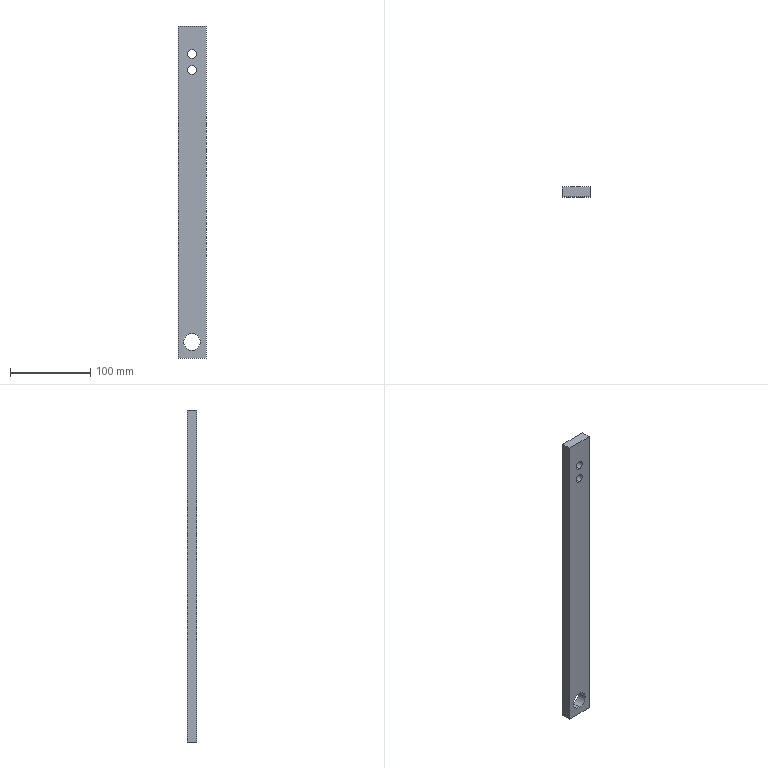Part | SolidWorks | features Extrusion 1, ICE 1 | 1 solid | 12 faces | box 35 x 12 x 415 mm | volume 167863 mm3 | cylinder 6 | plane 6 | commonest cylinder face diameters 11 x4 21 x2
STEP:
#1=CARTESIAN_POINT('',(0.,-6.,178.));
#2=VERTEX_POINT('',#1);
#3=CARTESIAN_POINT('',(0.,-6.,167.));
#4=VERTEX_POINT('',#3);
#5=CARTESIAN_POINT('',(0.,-6.,172.5));
#6=DIRECTION('',(0.,-1.,0.));
#7=DIRECTION('',(0.,0.,1.));
#8=AXIS2_PLACEMENT_3D('',#5,#6,#7);
#9=CIRCLE('',#8,5.5);
#10=EDGE_CURVE('',#2,#4,#9,.T.);
#11=ORIENTED_EDGE('',*,*,#10,.T.);
#12=CARTESIAN_POINT('',(0.,6.,167.));
#13=VERTEX_POINT('',#12);
#14=CARTESIAN_POINT('',(0.,-35.698,167.));
#15=DIRECTION('',(0.,1.,0.));
#16=VECTOR('',#15,1000.);
#17=LINE('',#14,#16);
#18=EDGE_CURVE('',#4,#13,#17,.T.);
#19=ORIENTED_EDGE('',*,*,#18,.T.);
#20=CARTESIAN_POINT('',(0.,6.,178.));
#21=VERTEX_POINT('',#20);
#22=CARTESIAN_POINT('',(0.,6.,172.5));
#23=DIRECTION('',(0.,1.,0.));
#24=DIRECTION('',(0.,0.,1.));
#25=AXIS2_PLACEMENT_3D('',#22,#23,#24);
#26=CIRCLE('',#25,5.5);
#27=EDGE_CURVE('',#13,#21,#26,.T.);
#28=ORIENTED_EDGE('',*,*,#27,.T.);
#29=CARTESIAN_POINT('',(0.,-35.698,178.));
#30=DIRECTION('',(0.,1.,0.));
#31=VECTOR('',#30,1000.);
#32=LINE('',#29,#31);
#33=EDGE_CURVE('',#2,#21,#32,.T.);
#34=ORIENTED_EDGE('',*,*,#33,.F.);
#35=EDGE_LOOP('',(#11,#19,#28,#34));
#36=FACE_OUTER_BOUND('',#35,.T.);
#37=CARTESIAN_POINT('',(0.,-35.698,172.5));
#38=DIRECTION('',(0.,1.,0.));
#39=DIRECTION('',(0.,0.,1.));
#40=AXIS2_PLACEMENT_3D('',#37,#38,#39);
#41=CYLINDRICAL_SURFACE('',#40,5.5);
#42=ADVANCED_FACE('',(#36),#41,.F.);
#43=CARTESIAN_POINT('',(0.,-6.,158.));
#44=VERTEX_POINT('',#43);
#45=CARTESIAN_POINT('',(0.,-6.,147.));
#46=VERTEX_POINT('',#45);
#47=CARTESIAN_POINT('',(0.,-6.,152.5));
#48=DIRECTION('',(0.,-1.,0.));
#49=DIRECTION('',(0.,0.,1.));
#50=AXIS2_PLACEMENT_3D('',#47,#48,#49);
#51=CIRCLE('',#50,5.5);
#52=EDGE_CURVE('',#44,#46,#51,.T.);
#53=ORIENTED_EDGE('',*,*,#52,.T.);
#54=CARTESIAN_POINT('',(0.,6.,147.));
#55=VERTEX_POINT('',#54);
#56=CARTESIAN_POINT('',(0.,-35.698,147.));
#57=DIRECTION('',(0.,1.,0.));
#58=VECTOR('',#57,1000.);
#59=LINE('',#56,#58);
#60=EDGE_CURVE('',#46,#55,#59,.T.);
#61=ORIENTED_EDGE('',*,*,#60,.T.);
#62=CARTESIAN_POINT('',(0.,6.,158.));
#63=VERTEX_POINT('',#62);
#64=CARTESIAN_POINT('',(0.,6.,152.5));
#65=DIRECTION('',(0.,1.,0.));
#66=DIRECTION('',(0.,0.,1.));
#67=AXIS2_PLACEMENT_3D('',#64,#65,#66);
#68=CIRCLE('',#67,5.5);
#69=EDGE_CURVE('',#55,#63,#68,.T.);
#70=ORIENTED_EDGE('',*,*,#69,.T.);
#71=CARTESIAN_POINT('',(0.,-35.698,158.));
#72=DIRECTION('',(0.,1.,0.));
#73=VECTOR('',#72,1000.);
#74=LINE('',#71,#73);
#75=EDGE_CURVE('',#44,#63,#74,.T.);
#76=ORIENTED_EDGE('',*,*,#75,.F.);
#77=EDGE_LOOP('',(#53,#61,#70,#76));
#78=FACE_OUTER_BOUND('',#77,.T.);
#79=CARTESIAN_POINT('',(0.,-35.698,152.5));
#80=DIRECTION('',(0.,1.,0.));
#81=DIRECTION('',(0.,0.,1.));
#82=AXIS2_PLACEMENT_3D('',#79,#80,#81);
#83=CYLINDRICAL_SURFACE('',#82,5.5);
#84=ADVANCED_FACE('',(#78),#83,.F.);
#85=CARTESIAN_POINT('',(0.,-6.,-177.));
#86=VERTEX_POINT('',#85);
#87=CARTESIAN_POINT('',(0.,-6.,-198.));
#88=VERTEX_POINT('',#87);
#89=CARTESIAN_POINT('',(0.,-6.,-187.5));
#90=DIRECTION('',(0.,-1.,0.));
#91=DIRECTION('',(0.,0.,1.));
#92=AXIS2_PLACEMENT_3D('',#89,#90,#91);
#93=CIRCLE('',#92,10.5);
#94=EDGE_CURVE('',#86,#88,#93,.T.);
#95=ORIENTED_EDGE('',*,*,#94,.T.);
#96=CARTESIAN_POINT('',(0.,6.,-198.));
#97=VERTEX_POINT('',#96);
#98=CARTESIAN_POINT('',(0.,-35.698,-198.));
#99=DIRECTION('',(0.,1.,0.));
#100=VECTOR('',#99,1000.);
#101=LINE('',#98,#100);
#102=EDGE_CURVE('',#88,#97,#101,.T.);
#103=ORIENTED_EDGE('',*,*,#102,.T.);
#104=CARTESIAN_POINT('',(0.,6.,-177.));
#105=VERTEX_POINT('',#104);
#106=CARTESIAN_POINT('',(0.,6.,-187.5));
#107=DIRECTION('',(0.,1.,0.));
#108=DIRECTION('',(0.,0.,1.));
#109=AXIS2_PLACEMENT_3D('',#106,#107,#108);
#110=CIRCLE('',#109,10.5);
#111=EDGE_CURVE('',#97,#105,#110,.T.);
#112=ORIENTED_EDGE('',*,*,#111,.T.);
#113=CARTESIAN_POINT('',(0.,-35.698,-177.));
#114=DIRECTION('',(0.,1.,0.));
#115=VECTOR('',#114,1000.);
#116=LINE('',#113,#115);
#117=EDGE_CURVE('',#86,#105,#116,.T.);
#118=ORIENTED_EDGE('',*,*,#117,.F.);
#119=EDGE_LOOP('',(#95,#103,#112,#118));
#120=FACE_OUTER_BOUND('',#119,.T.);
#121=CARTESIAN_POINT('',(0.,-35.698,-187.5));
#122=DIRECTION('',(0.,1.,0.));
#123=DIRECTION('',(0.,0.,1.));
#124=AXIS2_PLACEMENT_3D('',#121,#122,#123);
#125=CYLINDRICAL_SURFACE('',#124,10.5);
#126=ADVANCED_FACE('',(#120),#125,.F.);
#127=CARTESIAN_POINT('',(17.5,-6.,-207.5));
#128=VERTEX_POINT('',#127);
#129=CARTESIAN_POINT('',(17.5,6.,-207.5));
#130=VERTEX_POINT('',#129);
#131=CARTESIAN_POINT('',(17.5,-6.,-207.5));
#132=DIRECTION('',(0.,1.,0.));
#133=VECTOR('',#132,1000.);
#134=LINE('',#131,#133);
#135=EDGE_CURVE('',#128,#130,#134,.T.);
#136=ORIENTED_EDGE('',*,*,#135,.T.);
#137=CARTESIAN_POINT('',(17.5,6.,207.5));
#138=VERTEX_POINT('',#137);
#139=CARTESIAN_POINT('',(17.5,6.,207.5));
#140=DIRECTION('',(0.,0.,-1.));
#141=VECTOR('',#140,1000.);
#142=LINE('',#139,#141);
#143=EDGE_CURVE('',#138,#130,#142,.T.);
#144=ORIENTED_EDGE('',*,*,#143,.F.);
#145=CARTESIAN_POINT('',(17.5,-6.,207.5));
#146=VERTEX_POINT('',#145);
#147=CARTESIAN_POINT('',(17.5,-6.,207.5));
#148=DIRECTION('',(0.,1.,0.));
#149=VECTOR('',#148,1000.);
#150=LINE('',#147,#149);
#151=EDGE_CURVE('',#146,#138,#150,.T.);
#152=ORIENTED_EDGE('',*,*,#151,.F.);
#153=CARTESIAN_POINT('',(17.5,-6.,207.5));
#154=DIRECTION('',(0.,0.,-1.));
#155=VECTOR('',#154,1000.);
#156=LINE('',#153,#155);
#157=EDGE_CURVE('',#146,#128,#156,.T.);
#158=ORIENTED_EDGE('',*,*,#157,.T.);
#159=EDGE_LOOP('',(#136,#144,#152,#158));
#160=FACE_OUTER_BOUND('',#159,.T.);
#161=CARTESIAN_POINT('',(17.5,-6.,207.5));
#162=DIRECTION('',(-1.,0.,0.));
#163=DIRECTION('',(0.,0.,1.));
#164=AXIS2_PLACEMENT_3D('',#161,#162,#163);
#165=PLANE('',#164);
#166=ADVANCED_FACE('',(#160),#165,.F.);
#167=CARTESIAN_POINT('',(0.,6.,172.5));
#168=DIRECTION('',(0.,1.,0.));
#169=DIRECTION('',(0.,0.,1.));
#170=AXIS2_PLACEMENT_3D('',#167,#168,#169);
#171=CIRCLE('',#170,5.5);
#172=EDGE_CURVE('',#21,#13,#171,.T.);
#173=ORIENTED_EDGE('',*,*,#172,.F.);
#174=ORIENTED_EDGE('',*,*,#27,.F.);
#175=EDGE_LOOP('',(#173,#174));
#176=FACE_BOUND('',#175,.T.);
#177=CARTESIAN_POINT('',(0.,6.,152.5));
#178=DIRECTION('',(0.,1.,0.));
#179=DIRECTION('',(0.,0.,1.));
#180=AXIS2_PLACEMENT_3D('',#177,#178,#179);
#181=CIRCLE('',#180,5.5);
#182=EDGE_CURVE('',#63,#55,#181,.T.);
#183=ORIENTED_EDGE('',*,*,#182,.F.);
#184=ORIENTED_EDGE('',*,*,#69,.F.);
#185=EDGE_LOOP('',(#183,#184));
#186=FACE_BOUND('',#185,.T.);
#187=CARTESIAN_POINT('',(0.,6.,-187.5));
#188=DIRECTION('',(0.,1.,0.));
#189=DIRECTION('',(0.,0.,1.));
#190=AXIS2_PLACEMENT_3D('',#187,#188,#189);
#191=CIRCLE('',#190,10.5);
#192=EDGE_CURVE('',#105,#97,#191,.T.);
#193=ORIENTED_EDGE('',*,*,#192,.F.);
#194=ORIENTED_EDGE('',*,*,#111,.F.);
#195=EDGE_LOOP('',(#193,#194));
#196=FACE_BOUND('',#195,.T.);
#197=CARTESIAN_POINT('',(-17.5,6.,-207.5));
#198=VERTEX_POINT('',#197);
#199=CARTESIAN_POINT('',(-17.5,6.,-207.5));
#200=DIRECTION('',(-1.,0.,0.));
#201=VECTOR('',#200,1000.);
#202=LINE('',#199,#201);
#203=EDGE_CURVE('',#130,#198,#202,.T.);
#204=ORIENTED_EDGE('',*,*,#203,.T.);
#205=CARTESIAN_POINT('',(-17.5,6.,207.5));
#206=VERTEX_POINT('',#205);
#207=CARTESIAN_POINT('',(-17.5,6.,207.5));
#208=DIRECTION('',(0.,0.,-1.));
#209=VECTOR('',#208,1000.);
#210=LINE('',#207,#209);
#211=EDGE_CURVE('',#206,#198,#210,.T.);
#212=ORIENTED_EDGE('',*,*,#211,.F.);
#213=CARTESIAN_POINT('',(-17.5,6.,207.5));
#214=DIRECTION('',(-1.,0.,0.));
#215=VECTOR('',#214,1000.);
#216=LINE('',#213,#215);
#217=EDGE_CURVE('',#138,#206,#216,.T.);
#218=ORIENTED_EDGE('',*,*,#217,.F.);
#219=ORIENTED_EDGE('',*,*,#143,.T.);
#220=EDGE_LOOP('',(#204,#212,#218,#219));
#221=FACE_OUTER_BOUND('',#220,.T.);
#222=CARTESIAN_POINT('',(-17.5,6.,207.5));
#223=DIRECTION('',(0.,-1.,0.));
#224=DIRECTION('',(0.,0.,-1.));
#225=AXIS2_PLACEMENT_3D('',#222,#223,#224);
#226=PLANE('',#225);
#227=ADVANCED_FACE('',(#176,#186,#196,#221),#226,.F.);
#228=CARTESIAN_POINT('',(-17.5,-6.,-207.5));
#229=VERTEX_POINT('',#228);
#230=CARTESIAN_POINT('',(-17.5,-6.,-207.5));
#231=DIRECTION('',(0.,-1.,0.));
#232=VECTOR('',#231,1000.);
#233=LINE('',#230,#232);
#234=EDGE_CURVE('',#198,#229,#233,.T.);
#235=ORIENTED_EDGE('',*,*,#234,.T.);
#236=CARTESIAN_POINT('',(-17.5,-6.,207.5));
#237=VERTEX_POINT('',#236);
#238=CARTESIAN_POINT('',(-17.5,-6.,207.5));
#239=DIRECTION('',(0.,0.,-1.));
#240=VECTOR('',#239,1000.);
#241=LINE('',#238,#240);
#242=EDGE_CURVE('',#237,#229,#241,.T.);
#243=ORIENTED_EDGE('',*,*,#242,.F.);
#244=CARTESIAN_POINT('',(-17.5,-6.,207.5));
#245=DIRECTION('',(0.,-1.,0.));
#246=VECTOR('',#245,1000.);
#247=LINE('',#244,#246);
#248=EDGE_CURVE('',#206,#237,#247,.T.);
#249=ORIENTED_EDGE('',*,*,#248,.F.);
#250=ORIENTED_EDGE('',*,*,#211,.T.);
#251=EDGE_LOOP('',(#235,#243,#249,#250));
#252=FACE_OUTER_BOUND('',#251,.T.);
#253=CARTESIAN_POINT('',(-17.5,-6.,207.5));
#254=DIRECTION('',(1.,0.,0.));
#255=DIRECTION('',(0.,0.,-1.));
#256=AXIS2_PLACEMENT_3D('',#253,#254,#255);
#257=PLANE('',#256);
#258=ADVANCED_FACE('',(#252),#257,.F.);
#259=ORIENTED_EDGE('',*,*,#10,.F.);
#260=CARTESIAN_POINT('',(0.,-6.,172.5));
#261=DIRECTION('',(0.,-1.,0.));
#262=DIRECTION('',(0.,0.,1.));
#263=AXIS2_PLACEMENT_3D('',#260,#261,#262);
#264=CIRCLE('',#263,5.5);
#265=EDGE_CURVE('',#4,#2,#264,.T.);
#266=ORIENTED_EDGE('',*,*,#265,.F.);
#267=EDGE_LOOP('',(#259,#266));
#268=FACE_BOUND('',#267,.T.);
#269=ORIENTED_EDGE('',*,*,#52,.F.);
#270=CARTESIAN_POINT('',(0.,-6.,152.5));
#271=DIRECTION('',(0.,-1.,0.));
#272=DIRECTION('',(0.,0.,1.));
#273=AXIS2_PLACEMENT_3D('',#270,#271,#272);
#274=CIRCLE('',#273,5.5);
#275=EDGE_CURVE('',#46,#44,#274,.T.);
#276=ORIENTED_EDGE('',*,*,#275,.F.);
#277=EDGE_LOOP('',(#269,#276));
#278=FACE_BOUND('',#277,.T.);
#279=ORIENTED_EDGE('',*,*,#94,.F.);
#280=CARTESIAN_POINT('',(0.,-6.,-187.5));
#281=DIRECTION('',(0.,-1.,0.));
#282=DIRECTION('',(0.,0.,1.));
#283=AXIS2_PLACEMENT_3D('',#280,#281,#282);
#284=CIRCLE('',#283,10.5);
#285=EDGE_CURVE('',#88,#86,#284,.T.);
#286=ORIENTED_EDGE('',*,*,#285,.F.);
#287=EDGE_LOOP('',(#279,#286));
#288=FACE_BOUND('',#287,.T.);
#289=CARTESIAN_POINT('',(-17.5,-6.,-207.5));
#290=DIRECTION('',(1.,0.,0.));
#291=VECTOR('',#290,1000.);
#292=LINE('',#289,#291);
#293=EDGE_CURVE('',#229,#128,#292,.T.);
#294=ORIENTED_EDGE('',*,*,#293,.T.);
#295=ORIENTED_EDGE('',*,*,#157,.F.);
#296=CARTESIAN_POINT('',(-17.5,-6.,207.5));
#297=DIRECTION('',(1.,0.,0.));
#298=VECTOR('',#297,1000.);
#299=LINE('',#296,#298);
#300=EDGE_CURVE('',#237,#146,#299,.T.);
#301=ORIENTED_EDGE('',*,*,#300,.F.);
#302=ORIENTED_EDGE('',*,*,#242,.T.);
#303=EDGE_LOOP('',(#294,#295,#301,#302));
#304=FACE_OUTER_BOUND('',#303,.T.);
#305=CARTESIAN_POINT('',(-17.5,-6.,207.5));
#306=DIRECTION('',(0.,1.,0.));
#307=DIRECTION('',(0.,0.,1.));
#308=AXIS2_PLACEMENT_3D('',#305,#306,#307);
#309=PLANE('',#308);
#310=ADVANCED_FACE('',(#268,#278,#288,#304),#309,.F.);
#311=ORIENTED_EDGE('',*,*,#151,.T.);
#312=ORIENTED_EDGE('',*,*,#217,.T.);
#313=ORIENTED_EDGE('',*,*,#248,.T.);
#314=ORIENTED_EDGE('',*,*,#300,.T.);
#315=EDGE_LOOP('',(#311,#312,#313,#314));
#316=FACE_OUTER_BOUND('',#315,.T.);
#317=CARTESIAN_POINT('',(0.,0.,207.5));
#318=DIRECTION('',(0.,0.,-1.));
#319=DIRECTION('',(-1.,0.,0.));
#320=AXIS2_PLACEMENT_3D('',#317,#318,#319);
#321=PLANE('',#320);
#322=ADVANCED_FACE('',(#316),#321,.F.);
#323=ORIENTED_EDGE('',*,*,#135,.F.);
#324=ORIENTED_EDGE('',*,*,#293,.F.);
#325=ORIENTED_EDGE('',*,*,#234,.F.);
#326=ORIENTED_EDGE('',*,*,#203,.F.);
#327=EDGE_LOOP('',(#323,#324,#325,#326));
#328=FACE_OUTER_BOUND('',#327,.T.);
#329=CARTESIAN_POINT('',(0.,0.,-207.5));
#330=DIRECTION('',(0.,0.,-1.));
#331=DIRECTION('',(-1.,0.,0.));
#332=AXIS2_PLACEMENT_3D('',#329,#330,#331);
#333=PLANE('',#332);
#334=ADVANCED_FACE('',(#328),#333,.T.);
#335=ORIENTED_EDGE('',*,*,#102,.F.);
#336=ORIENTED_EDGE('',*,*,#285,.T.);
#337=ORIENTED_EDGE('',*,*,#117,.T.);
#338=ORIENTED_EDGE('',*,*,#192,.T.);
#339=EDGE_LOOP('',(#335,#336,#337,#338));
#340=FACE_OUTER_BOUND('',#339,.T.);
#341=CARTESIAN_POINT('',(0.,-35.698,-187.5));
#342=DIRECTION('',(0.,1.,0.));
#343=DIRECTION('',(0.,0.,1.));
#344=AXIS2_PLACEMENT_3D('',#341,#342,#343);
#345=CYLINDRICAL_SURFACE('',#344,10.5);
#346=ADVANCED_FACE('',(#340),#345,.F.);
#347=ORIENTED_EDGE('',*,*,#60,.F.);
#348=ORIENTED_EDGE('',*,*,#275,.T.);
#349=ORIENTED_EDGE('',*,*,#75,.T.);
#350=ORIENTED_EDGE('',*,*,#182,.T.);
#351=EDGE_LOOP('',(#347,#348,#349,#350));
#352=FACE_OUTER_BOUND('',#351,.T.);
#353=CARTESIAN_POINT('',(0.,-35.698,152.5));
#354=DIRECTION('',(0.,1.,0.));
#355=DIRECTION('',(0.,0.,1.));
#356=AXIS2_PLACEMENT_3D('',#353,#354,#355);
#357=CYLINDRICAL_SURFACE('',#356,5.5);
#358=ADVANCED_FACE('',(#352),#357,.F.);
#359=ORIENTED_EDGE('',*,*,#18,.F.);
#360=ORIENTED_EDGE('',*,*,#265,.T.);
#361=ORIENTED_EDGE('',*,*,#33,.T.);
#362=ORIENTED_EDGE('',*,*,#172,.T.);
#363=EDGE_LOOP('',(#359,#360,#361,#362));
#364=FACE_OUTER_BOUND('',#363,.T.);
#365=CARTESIAN_POINT('',(0.,-35.698,172.5));
#366=DIRECTION('',(0.,1.,0.));
#367=DIRECTION('',(0.,0.,1.));
#368=AXIS2_PLACEMENT_3D('',#365,#366,#367);
#369=CYLINDRICAL_SURFACE('',#368,5.5);
#370=ADVANCED_FACE('',(#364),#369,.F.);
#371=CLOSED_SHELL('',(#42,#84,#126,#166,#227,#258,#310,#322,#334,#346,#358,#370));
#372=MANIFOLD_SOLID_BREP('',#371);
#373=CARTESIAN_POINT('',(0.,0.,0.));
#374=DIRECTION('',(0.,0.,1.));
#375=DIRECTION('',(1.,0.,0.));
#376=AXIS2_PLACEMENT_3D('',#373,#374,#375);
#377=(LENGTH_UNIT()NAMED_UNIT(*)SI_UNIT(.MILLI.,.METRE.));
#378=UNCERTAINTY_MEASURE_WITH_UNIT(LENGTH_MEASURE(0.00001),#377,'','');
#379=(NAMED_UNIT(*)PLANE_ANGLE_UNIT()SI_UNIT($,.RADIAN.));
#380=(NAMED_UNIT(*)SI_UNIT($,.STERADIAN.)SOLID_ANGLE_UNIT());
#381=(GEOMETRIC_REPRESENTATION_CONTEXT(3)GLOBAL_UNCERTAINTY_ASSIGNED_CONTEXT((#378))GLOBAL_UNIT_ASSIGNED_CONTEXT((#377,#379,#380))REPRESENTATION_CONTEXT('',''));
#382=ADVANCED_BREP_SHAPE_REPRESENTATION('',(#372,#376),#381);